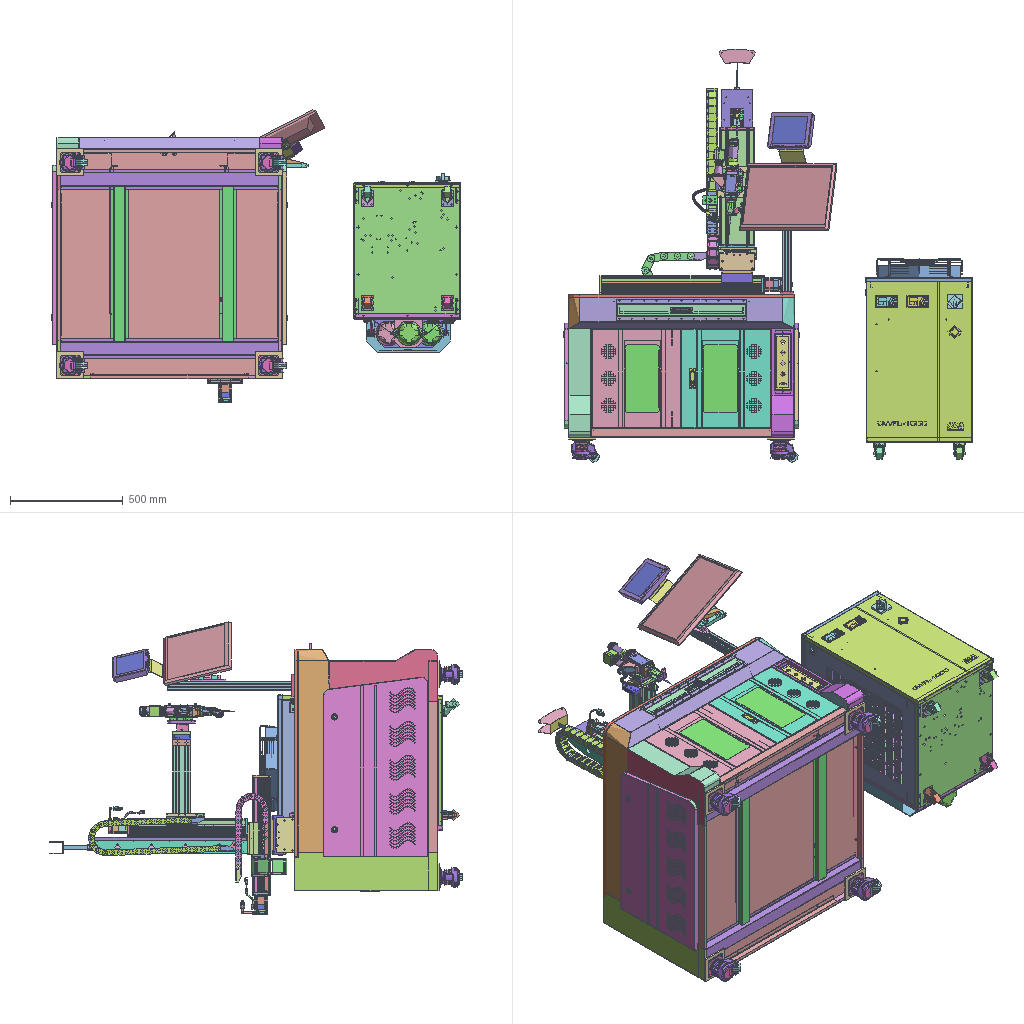Assembly | STEP file | 293 different items | 588 placed | box 1817 x 1832 x 1296 mm
Parts list (item | name | quantity | parent item | size | volume):
1 | FHD-021-001-A rack welded part A | x1 | in BHB-002-000-001 rack welding | 1000 x 1020 x 40 mm | 1755209 mm3
2 | FHD-021-001-B rack welded part B | x1 | in BHB-002-000-001 rack welding | 1000 x 198.5 x 167.5 mm | 523284 mm3
3 | FHD-021-001-C rack welded part C | x1 | in BHB-002-000-001 rack welding | 633.5 x 171.5 x 165 mm | 350229 mm3
4 | FHD-021-001-D rack welded part D | x1 | in BHB-002-000-001 rack welding | 633.5 x 165 x 171.5 mm | 312915 mm3
5 | FHD-021-001-E rack welded part E | x1 | in BHB-002-000-001 rack welding | 900 x 139 x 50 mm | 280758 mm3
6 | FHD-021-001-F rack welded part F | x1 | in BHB-002-000-001 rack welding | 900 x 139 x 50 mm | 288308 mm3
7 | FHD-021-001-G rack welded part G | x1 | in BHB-002-000-001 rack welding | 1000 x 178.631 x 144.83 mm | 461158 mm3
8 | FHD-021-001-H rack welded part H | x1 | in BHB-002-000-001 rack welding | 483 x 230 x 20 mm | 162335 mm3
9 | FHD-021-001-I rack welded part I | x1 | in BHB-002-000-001 rack welding | 483 x 230 x 20 mm | 162335 mm3
10 | FHD-021-001-J rack welded part J | x1 | in BHB-002-000-001 rack welding | 482.9 x 130.5 x 173 mm | 174985 mm3
11 | FHD-021-001-K rack welded part K | x1 | in BHB-002-000-001 rack welding | 482.9 x 126.5 x 173 mm | 173847 mm3
12 | FHD-021-001-L rack welded part L | x1 | in BHB-002-000-001 rack welding | 480.9 x 65 x 100 mm | 53460 mm3
13 | FHD-021-001-M rack welded part M | x1 | in BHB-002-000-001 rack welding | 480.9 x 65 x 100 mm | 79687 mm3
14 | FHD-021-001-N rack welded part N | x2 | in BHB-002-000-001 rack welding | 30 x 73.5 x 446.5 mm | 80480 mm3
15 | FHD-021-001-O rack welded part O | x2 | in BHB-002-000-001 rack welding | 20 x 73.5 x 446.5 mm | 91052 mm3
16 | FHD-021-001-P rack welded part P | x2 | in BHB-002-000-001 rack welding | 1000 x 80 x 15 mm | 159142 mm3
17 | FHD-021-001-Q rack welded part Q | x1 | in BHB-002-000-001 rack welding | 280 x 73 x 20 mm | 29608 mm3
18 | FHD-021-001-R rack welded part R | x1 | in BHB-002-000-001 rack welding | 244 x 74 x 1.5 mm | 11328 mm3
19 | FHD-021-001-Z Fuma wheel mounting plate | x4 | in BHB-002-000-001 rack welding | 120 x 120 x 8 mm | 114038 mm3
20 | FHD-021-001-S rack welded part S | x2 | in BHB-002-000-001 rack welding | 969 x 87 x 38.5 mm | 231643 mm3
21 | FHD-021-001-T rack welded part T | x2 | in BHB-002-000-001 rack welding | 690 x 77 x 20 mm | 115059 mm3
22 | FHD-021-001-U rack welded part U | x1 | in BHB-002-000-001 rack welding | 336.5 x 121.5 x 15 mm | 72345 mm3
23 | FHD-021-001-V rack welded part V | x1 | in BHB-002-000-001 rack welding | 336.5 x 121.5 x 15 mm | 72345 mm3
24 | FHD-021-001-W rack welded part W | x2 | in BHB-002-000-001 rack welding | 575 x 20 x 15 mm | 28039 mm3
25 | FHD-021-001-X rack welded part X | x1 | in BHB-002-000-001 rack welding | 143 x 80 x 15 mm | 22271 mm3
26 | FHD-021-001-Y rack welded part Y | x1 | in BHB-002-000-001 rack welding | 146 x 60 x 15 mm | 27524 mm3
27 | FHD-021-002 electrical mounting plate | x2 | in FHD-021-000 H1010 cabinet | 650 x 440 x 15 mm | 470822 mm3
28 | FHD-021-003 rear door lower crossbeam | x1 | in FHD-021-000 H1010 cabinet | 695 x 103 x 22 mm | 152226 mm3
29 | FHD-021-004-A rear door A | x1 | in FHD-021-004 rear door welded body | 693 x 376 x 18 mm | 424515 mm3
30 | FHD-021-004-B fan support cover | x4 | in FHD-021-004 rear door welded body | 139 x 132 x 7 mm | 12460 mm3
31 | FHD-021-004-C rear door reinforcing rib | x1 | in FHD-021-004 rear door welded body | 348 x 57 x 10 mm | 37777 mm3
32 | FHD-021-005 power button plate | x1 | in FHD-021-000 H1010 cabinet | 248 x 68 x 1.5 mm | 22504 mm3
33 | FHD-021-006 rear power board | x1 | in FHD-021-000 H1010 cabinet | 228.5 x 58.5 x 3.2 mm | 14630 mm3
34 | FHD-021-007-A TZD10S drawer 1 | x1 | in FHD-021-007 TZD10S drawer assembly | 569.6 x 52 x 18 mm | 67956 mm3
35 | FHD-021-007-B TZD10S drawer 2 | x1 | in FHD-021-007 TZD10S drawer assembly | 548 x 320 x 25 mm | 247788 mm3
36 | FHD-021-007-C TZD10S drawer 3 | x2 | in FHD-021-007 TZD10S drawer assembly | 52 x 18 x 12 mm | 1523 mm3
37 | FHD-021-007-D TZD10S drawer 4 | x1 | in FHD-021-007 TZD10S drawer assembly | 150 x 90 x 35 mm | 35026 mm3
38 | LS707 rotary concealed handle | x2 | in FHD-021-007 TZD10S drawer assembly, FHD-021-000 H1010 cabinet | 63.292 x 100 x 20 mm | 9779 mm3
39 | FHD-021-008-01-A circuit breaker bracket 1 | x1 | in FHD-021-008-01 circuit breaker bracket welding | 100 x 108 x 20 mm | 20485 mm3
40 | FHD-021-008-01-B circuit breaker bracket 2 | x2 | in FHD-021-008-01 circuit breaker bracket welding | 57 x 47 x 15 mm | 5499 mm3
41 | FHD-021-008-01-C circuit breaker bracket 3 | x2 | in FHD-021-008-01 circuit breaker bracket welding | 76 x 20 x 1.5 mm | 2280 mm3
42 | FHD-021-008-02 limit block | x2 | in FHD-021-008 circuit breaker assembly | 60 x 70 x 19 mm | 6672 mm3
43 | FHD-021-008-03 fixing plate | x1 | in FHD-021-008 circuit breaker assembly | 103 x 25 x 1.5 mm | 3776 mm3
44 | FHD-021-009 front baffle | x2 | in FHD-021-000 H1010 cabinet | 215 x 35 x 2 mm | 14477 mm3
45 | door lock catch | x2 | in MS603 red spring door lock, MS603 red spring door lock_2 | 26.4 x 86 x 16.7 mm | 21050 mm3
46 | door lock bent plate | x2 | in MS603 red spring door lock, MS603 red spring door lock_2 | 65.681 x 31 x 12.394 mm | 2703 mm3
47 | slide rail 300-1 | x2 | in 12-inch silent slide rail, 12-inch silent slide rail_2 | 300 x 46.341 x 13 mm | 22910 mm3
48 | slide rail 300-2 | x2 | in 12-inch silent slide rail, 12-inch silent slide rail_2 | 10.373 x 34.385 x 300 mm | 15280 mm3
49 | slide rail 300-3 | x2 | in 12-inch silent slide rail, 12-inch silent slide rail_2 | 9.001 x 23.751 x 300 mm | 9128 mm3
50 | FHD-021-010 L-shaped support rail | x1 | in FHD-021-000 H1010 cabinet | 620 x 30 x 50 mm | 94894 mm3
51 | FHD-021-011-A side door A | x1 | in FHD-021-011 side door A welded body | 795.88 x 474.5 x 40 mm | 624851 mm3
52 | FHD-021-012-B side door A-B | x2 | in FHD-021-011 side door A welded body, FHD-021-012 side door B welded body | 29.753 x 26.353 x 17 mm | 1076 mm3
53 | FHD-021-012-C side door A-C | x2 | in FHD-021-011 side door A welded body, FHD-021-012 side door B welded body | 30 x 33.839 x 17 mm | 1267 mm3
54 | FHD-021-012-D side door A-D | x2 | in FHD-021-011 side door A welded body, FHD-021-012 side door B welded body | 29.753 x 27.697 x 1.5 mm | 623.148 mm3
55 | FHD-021-012-F side door A-E | x2 | in FHD-021-011 side door A welded body, FHD-021-012 side door B welded body | 30 x 33.839 x 1.5 mm | 734.02 mm3
56 | FHD-0210-012-E side door A-F | x2 | in FHD-021-011 side door A welded body, FHD-021-012 side door B welded body | 757 x 71 x 12 mm | 102614 mm3
57 | FHD-021-012-A side door B | x1 | in FHD-021-012 side door B welded body | 795.88 x 474.5 x 40 mm | 624852 mm3
58 | FHD-021-013-A front door A | x1 | in FHD-021-013-01 front door A welding | 397 x 457.5 x 17.5 mm | 250425 mm3
59 | FHD-021-014-C acrylic mounting strip | x4 | in FHD-021-013-01 front door A welding, FHD-021-014-01 front door B welding | 430 x 20 x 10 mm | 23632 mm3
60 | FHD-021-014-02 acrylic press plate | x4 | in FHD-021-013 front door A, FHD-021-014 front door B welded body | 250 x 28 x 7 mm | 12276 mm3
61 | FHD-021-014-03 acrylic | x2 | in FHD-021-013 front door A, FHD-021-014 front door B welded body | 385 x 160 x 5 mm | 308000 mm3
62 | FHD-021-014-A front door B | x1 | in FHD-021-014-01 front door B welding | 410 x 447 x 20 mm | 253871 mm3
63 | FHD-021-014-B latch mounting seat | x2 | in FHD-021-014-01 front door B welding | 70 x 40 x 15 mm | 6920 mm3
64 | latch | x2 | in LS406 automatic spring latch, LS406 automatic spring latch_2 | 30 x 13 x 66 mm | 12946 mm3
65 | latch post | x2 | in LS406 automatic spring latch, LS406 automatic spring latch_2 | 16 x 83 x 14 mm | 4581 mm3
66 | MS705-18 triangular lock core | x4 | in FHD-021-000 H1010 cabinet | 28 x 32 x 60.591 mm | 12821 mm3
67 | FHD-021-015 H1010 revised work panel | x1 | in FHD-021-000 H1010 cabinet | 1000 x 918 x 15 mm | 13697706 mm3
68 | - | x4 | in GD-80-F Fuma(2)^GD-80-F Fuma, GD-80-F Fuma(2)^GD-80-F Fuma_2, GD-80-F Fuma(2)^GD-80-F Fuma_3, GD-80-F Fuma(2)^GD-80-F Fuma_4 | 9.62 x 9.62 x 8 mm | 49.009 mm3
69 | - | x4 | in GD-80-F Fuma(2)^GD-80-F Fuma, GD-80-F Fuma(2)^GD-80-F Fuma_2, GD-80-F Fuma(2)^GD-80-F Fuma_3, GD-80-F Fuma(2)^GD-80-F Fuma_4 | 7.817 x 18 x 5 mm | 4.038 mm3
70 | - | x4 | in GD-80-F Fuma(2)^GD-80-F Fuma, GD-80-F Fuma(2)^GD-80-F Fuma_2, GD-80-F Fuma(2)^GD-80-F Fuma_3, GD-80-F Fuma(2)^GD-80-F Fuma_4 | 90 x 90 x 88.64 mm | 185053 mm3
71 | - | x4 | in GD-80-F Fuma(2)^GD-80-F Fuma, GD-80-F Fuma(2)^GD-80-F Fuma_2, GD-80-F Fuma(2)^GD-80-F Fuma_3, GD-80-F Fuma(2)^GD-80-F Fuma_4 | 63 x 32 x 63 mm | 83090 mm3
72 | - | x4 | in GD-80-F Fuma(2)^GD-80-F Fuma, GD-80-F Fuma(2)^GD-80-F Fuma_2, GD-80-F Fuma(2)^GD-80-F Fuma_3, GD-80-F Fuma(2)^GD-80-F Fuma_4 | 27.164 x 61.45 x 3.959 mm | 161.362 mm3
73 | - | x4 | in GD-80-F Fuma(2)^GD-80-F Fuma, GD-80-F Fuma(2)^GD-80-F Fuma_2, GD-80-F Fuma(2)^GD-80-F Fuma_3, GD-80-F Fuma(2)^GD-80-F Fuma_4 | 110.5 x 86 x 80.5 mm | 156144 mm3
74 | - | x1 | - | 3 x 5.5 x 5.5 mm | 47.924 mm3
75 | - | x1 | - | 6 x 6 x 0.5 mm | 10.116 mm3
76 | - | x1 | - | 3 x 5.5 x 5.5 mm | 47.924 mm3
77 | - | x1 | - | 6 x 6 x 0.5 mm | 10.116 mm3
78 | - | x1 | - | 3 x 5.5 x 5.5 mm | 47.924 mm3
79 | - | x1 | - | 6 x 6 x 0.5 mm | 10.116 mm3
80 | - | x1 | - | 3 x 5.5 x 5.5 mm | 47.924 mm3
81 | - | x1 | - | 6 x 6 x 0.5 mm | 10.116 mm3
82 | - | x1 | - | 3 x 5.5 x 5.5 mm | 47.924 mm3
83 | - | x1 | - | 6 x 6 x 0.5 mm | 10.116 mm3
84 | - | x1 | - | 3 x 5.5 x 5.5 mm | 47.924 mm3
85 | - | x1 | - | 6 x 6 x 0.5 mm | 10.116 mm3
86 | - | x1 | - | 3 x 5.5 x 5.5 mm | 47.924 mm3
87 | - | x1 | - | 6 x 6 x 0.5 mm | 10.116 mm3
88 | - | x1 | - | 3 x 5.5 x 5.5 mm | 47.924 mm3
89 | - | x1 | - | 6 x 6 x 0.5 mm | 10.116 mm3
90 | - | x1 | - | 2.7 x 4.5 x 4.5 mm | 28.373 mm3
91 | - | x1 | - | 5.2 x 5.179 x 0.6 mm | 8.765 mm3
92 | - | x1 | - | 5 x 5 x 0.5 mm | 6.955 mm3
93 | - | x1 | - | 2.7 x 4.5 x 4.5 mm | 28.373 mm3
94 | - | x1 | - | 5.2 x 5.179 x 0.6 mm | 8.765 mm3
95 | - | x1 | - | 5 x 5 x 0.5 mm | 6.955 mm3
96 | - | x1 | - | 60 x 60 x 34.1 mm | 106428 mm3
97 | - | x1 | - | 59.4 x 59.4 x 23.3 mm | 72108 mm3
98 | - | x1 | - | 60 x 60 x 6.4 mm | 20143 mm3
99 | - | x1 | - | 59.8 x 59.8 x 0.5 mm | 1478 mm3
100 | - | x1 | - | 59.8 x 64.9 x 13.2 mm | 38412 mm3
101 | - | x1 | - | 30 x 8.8 x 21 mm | 202.601 mm3
102 | - | x1 | - | 30 x 12.5 x 21 mm | 6057 mm3
103 | - | x1 | - | 10.4 x 42.4 x 119.7 mm | 5288 mm3
104 | - | x1 | - | 58.9 x 42.4 x 59.5 mm | 11878 mm3
105 | - | x1 | - | 10.6 x 6.6 x 10.6 mm | 286.348 mm3
106 | - | x1 | - | 13.2 x 8.2 x 13.2 mm | 283.542 mm3
107 | - | x1 | - | 60.2 x 60.2 x 9.5 mm | 18131 mm3
108 | - | x1 | - | 35 x 10 x 35 mm | 6585 mm3
109 | - | x1 | - | 17 x 17 x 80.2 mm | 12671 mm3
110 | - | x4 | - | 2.5 x 2.5 x 10 mm | 49.087 mm3
111 | - | x1 | - | 5 x 5 x 14 mm | 350 mm3
112 | - | x1 | - | 155 x 59.25 x 710 mm | 2291681 mm3
113 | - | x1 | - | 170 x 42.5 x 140 mm | 521938 mm3
114 | - | x1 | - | 155 x 25 x 709.4 mm | 387813 mm3
115 | - | x1 | - | 49 x 39.6 x 50 mm | 57288 mm3
116 | - | x1 | - | 155 x 82 x 12 mm | 118532 mm3
117 | - | x1 | - | 155 x 82 x 10 mm | 121887 mm3
118 | - | x2 | - | 15 x 15 x 700 mm | 150376 mm3
119 | - | x1 | - | 69.5 x 46 x 22 mm | 45024 mm3
120 | - | x1 | - | 69.5 x 49 x 25 mm | 41553 mm3
121 | - | x1 | - | 16 x 16 x 675 mm | 128698 mm3
122 | - | x4 | - | 56 x 33 x 16 mm | 20352 mm3
123 | - | x1 | - | 40 x 30 x 10 mm | 9671 mm3
124 | - | x1 | in X-axis module | 170 x 140 x 12 mm | 282154 mm3
125 | - | x2 | in module drag chain72X35assemblyX500 stroke | 104 x 72 x 35 mm | 42394 mm3
126 | - | x14 | in module drag chain72X35assemblyX500 stroke | 94 x 35 x 72 mm | 47784 mm3
127 | - | x1 | - | 15 x 15 x 500 mm | 107236 mm3
128 | - | x2 | - | 56 x 33 x 16 mm | 20352 mm3
129 | - | x1 | - | 15 x 15 x 500 mm | 107236 mm3
130 | - | x2 | - | 56 x 33 x 16 mm | 20352 mm3
131 | - | x1 | - | 3 x 5.5 x 5.5 mm | 47.924 mm3
132 | - | x1 | - | 6 x 6 x 0.5 mm | 10.116 mm3
133 | - | x1 | - | 3 x 5.5 x 5.5 mm | 47.924 mm3
134 | - | x1 | - | 6 x 6 x 0.5 mm | 10.116 mm3
135 | - | x1 | - | 3 x 5.5 x 5.5 mm | 47.924 mm3
136 | - | x1 | - | 6 x 6 x 0.5 mm | 10.116 mm3
137 | - | x1 | - | 3 x 5.5 x 5.5 mm | 47.924 mm3
138 | - | x1 | - | 6 x 6 x 0.5 mm | 10.116 mm3
139 | - | x1 | - | 3 x 5.5 x 5.5 mm | 47.924 mm3
140 | - | x1 | - | 6 x 6 x 0.5 mm | 10.116 mm3
141 | - | x1 | - | 3 x 5.5 x 5.5 mm | 47.924 mm3
142 | - | x1 | - | 6 x 6 x 0.5 mm | 10.116 mm3
143 | - | x1 | - | 3 x 5.5 x 5.5 mm | 47.924 mm3
144 | - | x1 | - | 6 x 6 x 0.5 mm | 10.116 mm3
145 | - | x1 | - | 3 x 5.5 x 5.5 mm | 47.924 mm3
146 | - | x1 | - | 6 x 6 x 0.5 mm | 10.116 mm3
147 | - | x1 | - | 2.7 x 4.5 x 4.5 mm | 28.373 mm3
148 | - | x1 | - | 5.2 x 5.179 x 0.6 mm | 8.765 mm3
149 | - | x1 | - | 5 x 5 x 0.5 mm | 6.955 mm3
150 | - | x1 | - | 2.7 x 4.5 x 4.5 mm | 28.373 mm3
151 | - | x1 | - | 5.2 x 5.179 x 0.6 mm | 8.765 mm3
152 | - | x1 | - | 5 x 5 x 0.5 mm | 6.955 mm3
153 | - | x1 | - | 60 x 60 x 34.1 mm | 106428 mm3
154 | - | x1 | - | 59.4 x 59.4 x 23.3 mm | 72108 mm3
155 | - | x1 | - | 60 x 60 x 6.4 mm | 20143 mm3
156 | - | x1 | - | 59.8 x 59.8 x 0.5 mm | 1478 mm3
157 | - | x1 | - | 59.8 x 64.9 x 13.2 mm | 38412 mm3
158 | - | x1 | - | 30 x 8.8 x 21 mm | 202.601 mm3
159 | - | x1 | - | 30 x 12.5 x 21 mm | 6057 mm3
160 | - | x1 | - | 10.4 x 42.4 x 119.7 mm | 5288 mm3
161 | - | x1 | - | 58.9 x 42.4 x 59.5 mm | 11878 mm3
162 | - | x1 | - | 10.6 x 6.6 x 10.6 mm | 286.348 mm3
163 | - | x1 | - | 13.2 x 8.2 x 13.2 mm | 283.542 mm3
164 | - | x1 | - | 60.2 x 60.2 x 9.5 mm | 18131 mm3
165 | - | x1 | - | 35 x 10 x 35 mm | 6585 mm3
166 | - | x1 | - | 17 x 17 x 80.2 mm | 12671 mm3
167 | - | x4 | - | 2.5 x 2.5 x 10 mm | 49.087 mm3
168 | - | x1 | - | 5 x 5 x 14 mm | 350 mm3
169 | - | x1 | - | 475 x 15 x 15 mm | 78728 mm3
170 | - | x1 | - | 10 x 15 x 15 mm | 632.723 mm3
171 | - | x1 | - | 38 x 48 x 40 mm | 23611 mm3
172 | - | x1 | - | 155 x 59.25 x 510 mm | 1638081 mm3
173 | - | x1 | - | 49 x 39.6 x 50 mm | 57288 mm3
174 | - | x1 | - | 170 x 42.5 x 140 mm | 522527 mm3
175 | - | x1 | - | 155 x 25 x 509.4 mm | 278478 mm3
176 | - | x1 | - | 155 x 82 x 12 mm | 118532 mm3
177 | - | x1 | - | 155 x 82 x 10 mm | 121887 mm3
178 | - | x1 | - | 69.5 x 46 x 22 mm | 45024 mm3
179 | - | x1 | - | 69.5 x 49 x 25 mm | 41553 mm3
180 | - | x1 | - | 38 x 11 x 30 mm | 9809 mm3
181 | - | x2 | - | 12 x 14 x 12 mm | 1266 mm3
182 | - | x1 | - | 8 x 26 x 26 mm | 3460 mm3
183 | - | x1 | - | 54 x 54 x 34.8 mm | 31485 mm3
184 | - | x1 | - | 28 x 28 x 32 mm | 13816 mm3
185 | - | x1 | - | 5 x 11.9 x 37.5 mm | 433.441 mm3
186 | - | x2 | - | 13.4 x 41 x 12 mm | 1188 mm3
187 | - | x48 | - | 20 x 7 x 7 mm | 335.507 mm3
188 | - | x10 | - | 21 x 8.5 x 8.5 mm | 554.949 mm3
189 | - | x4 | - | 11 x 5.5 x 5.5 mm | 118.766 mm3
190 | - | x16 | - | 25 x 8.5 x 8.5 mm | 633.488 mm3
191 | - | x1 | - | 12.9 x 14.3 x 1 mm | 65.231 mm3
192 | - | x1 | in Y-axis module | 300 x 60 x 32 mm | 62070 mm3
193 | - | x1 | in Y-axis module | 100 x 72 x 35 mm | 19846 mm3
194 | - | x2 | - | 80 x 48 x 25 mm | 22611 mm3
195 | - | x17 | - | 58.5 x 25 x 48 mm | 18741 mm3
196 | - | x2 | - | 60 x 700 x 15 mm | 546170 mm3
197 | - | x1 | - | 170 x 140 x 12 mm | 277366 mm3
198 | - | x1 | - | 700 x 140 x 15 mm | 1462585 mm3
199 | - | x1 | - | 60 x 58 x 60 mm | 38921 mm3
200 | - | x2 | - | 1.5 x 159.863 x 63.96 mm | 12341 mm3
201 | - | x1 | - | 20 x 20 x 700 mm | 96209 mm3
202 | - | x1 | - | 50 x 106.693 x 5.46 mm | 7969 mm3
203 | - | x1 | - | 28 x 25 x 700 mm | 101372 mm3
204 | - | x1 | - | 15 x 15 x 500 mm | 107236 mm3
205 | - | x2 | - | 56 x 33 x 16 mm | 20352 mm3
206 | - | x1 | - | 15 x 15 x 500 mm | 107236 mm3
207 | - | x2 | - | 56 x 33 x 16 mm | 20352 mm3
208 | - | x1 | - | 3 x 5.5 x 5.5 mm | 47.924 mm3
209 | - | x1 | - | 6 x 6 x 0.5 mm | 10.116 mm3
210 | - | x1 | - | 3 x 5.5 x 5.5 mm | 47.924 mm3
211 | - | x1 | - | 6 x 6 x 0.5 mm | 10.116 mm3
212 | - | x1 | - | 3 x 5.5 x 5.5 mm | 47.924 mm3
213 | - | x1 | - | 6 x 6 x 0.5 mm | 10.116 mm3
214 | - | x1 | - | 3 x 5.5 x 5.5 mm | 47.924 mm3
215 | - | x1 | - | 6 x 6 x 0.5 mm | 10.116 mm3
216 | - | x1 | - | 3 x 5.5 x 5.5 mm | 47.924 mm3
217 | - | x1 | - | 6 x 6 x 0.5 mm | 10.116 mm3
218 | - | x1 | - | 3 x 5.5 x 5.5 mm | 47.924 mm3
219 | - | x1 | - | 6 x 6 x 0.5 mm | 10.116 mm3
220 | - | x1 | - | 3 x 5.5 x 5.5 mm | 47.924 mm3
221 | - | x1 | - | 6 x 6 x 0.5 mm | 10.116 mm3
222 | - | x1 | - | 3 x 5.5 x 5.5 mm | 47.924 mm3
223 | - | x1 | - | 6 x 6 x 0.5 mm | 10.116 mm3
224 | - | x1 | - | 2.7 x 4.5 x 4.5 mm | 28.373 mm3
225 | - | x1 | - | 5.2 x 5.179 x 0.6 mm | 8.765 mm3
226 | - | x1 | - | 5 x 5 x 0.5 mm | 6.955 mm3
227 | - | x1 | - | 2.7 x 4.5 x 4.5 mm | 28.373 mm3
228 | - | x1 | - | 5.2 x 5.179 x 0.6 mm | 8.765 mm3
229 | - | x1 | - | 5 x 5 x 0.5 mm | 6.955 mm3
230 | - | x1 | - | 60 x 60 x 34.1 mm | 106428 mm3
231 | - | x1 | - | 59.4 x 59.4 x 23.3 mm | 72108 mm3
232 | - | x1 | - | 60 x 60 x 6.4 mm | 20143 mm3
233 | - | x1 | - | 59.8 x 59.8 x 0.5 mm | 1478 mm3
234 | - | x1 | - | 59.8 x 64.9 x 13.2 mm | 38412 mm3
235 | - | x1 | - | 30 x 8.8 x 21 mm | 202.601 mm3
236 | - | x1 | - | 30 x 12.5 x 21 mm | 6057 mm3
237 | - | x1 | - | 10.4 x 42.4 x 119.7 mm | 5288 mm3
238 | - | x1 | - | 58.9 x 42.4 x 59.5 mm | 11878 mm3
239 | - | x1 | - | 10.6 x 6.6 x 10.6 mm | 286.348 mm3
240 | - | x1 | - | 13.2 x 8.2 x 13.2 mm | 283.542 mm3
241 | - | x1 | - | 60.2 x 60.2 x 9.5 mm | 18131 mm3
242 | - | x1 | - | 35 x 10 x 35 mm | 6585 mm3
243 | - | x1 | - | 17 x 17 x 80.2 mm | 12671 mm3
244 | - | x4 | - | 2.5 x 2.5 x 10 mm | 49.087 mm3
245 | - | x1 | - | 5 x 5 x 14 mm | 350 mm3
246 | - | x1 | - | 475 x 15 x 15 mm | 78728 mm3
247 | - | x1 | - | 10 x 15 x 15 mm | 632.723 mm3
248 | - | x1 | - | 38 x 48 x 40 mm | 23611 mm3
249 | - | x1 | - | 155 x 59.25 x 510 mm | 1638081 mm3
250 | - | x1 | - | 49 x 39.6 x 50 mm | 57288 mm3
251 | - | x1 | - | 170 x 42.5 x 140 mm | 522527 mm3
252 | - | x1 | - | 155 x 25 x 509.4 mm | 278478 mm3
253 | - | x1 | - | 155 x 82 x 12 mm | 118532 mm3
254 | - | x1 | - | 155 x 82 x 10 mm | 121887 mm3
255 | - | x1 | - | 69.5 x 46 x 22 mm | 45024 mm3
256 | - | x1 | - | 69.5 x 49 x 25 mm | 41553 mm3
257 | - | x1 | - | 38 x 11 x 30 mm | 9809 mm3
258 | - | x2 | - | 12 x 14 x 12 mm | 1266 mm3
259 | - | x1 | - | 8 x 26 x 26 mm | 3460 mm3
260 | - | x1 | - | 54 x 54 x 34.8 mm | 31485 mm3
261 | - | x1 | - | 28 x 28 x 32 mm | 13816 mm3
262 | - | x1 | - | 5 x 11.9 x 37.5 mm | 433.441 mm3
263 | - | x2 | - | 13.4 x 41 x 12 mm | 1188 mm3
264 | - | x48 | - | 20 x 7 x 7 mm | 335.507 mm3
265 | - | x10 | - | 21 x 8.5 x 8.5 mm | 554.949 mm3
266 | - | x4 | - | 11 x 5.5 x 5.5 mm | 118.766 mm3
267 | - | x16 | - | 25 x 8.5 x 8.5 mm | 633.488 mm3
268 | - | x1 | - | 12.9 x 14.3 x 1 mm | 65.231 mm3
269 | - | x1 | - | 80 x 80 x 350 mm | 477520 mm3
270 | - | x1 | - | 80 x 50 x 14 mm | 51452 mm3
271 | - | x1 | - | 80 x 40 x 20 mm | 53799 mm3
272 | - | x1 | - | 80 x 80 x 15 mm | 88507 mm3
273 | - | x1 | - | 58 x 50 x 30 mm | 56140 mm3
274 | - | x1 | - | 36 x 36 x 35 mm | 25571 mm3
275 | - | x1 | - | 170 x 140 x 12 mm | 277063 mm3
276 | - | x1 | - | 120 x 90 x 12 mm | 121667 mm3
277 | - | x1 | in Z-axis module | 68 x 40 x 15 mm | 6435 mm3
278 | - | x1 | in Z-axis module | 76 x 36 x 47 mm | 12306 mm3
279 | module 48X25 drag chainA | x2 | in module 48X25 drag chainB | 80 x 48 x 25 mm | 22611 mm3
280 | module 48X25 drag chainA2 | x32 | in module 48X25 drag chainB | 58.5 x 25 x 48 mm | 18741 mm3
281 | XHG200AYH(F100-F200) | x1 | in welding head moving assembly | - | -
282 | - | x1 | - | 60.601 x 162 x 27 mm | 75887 mm3
283 | - | x2 | - | 20 x 160 x 29 mm | 68270 mm3
284 | - | x1 | - | 128 x 18 x 30 mm | 60581 mm3
285 | - | x1 | - | 41.5 x 23 x 23 mm | 10947 mm3
286 | - | x1 | - | 116 x 116 x 45 mm | 39889 mm3
287 | - | x1 | in monitor stand BPB-037-000 monitor column mounting assembly(2)^BPB-037-000 monitor column mounting assembly | 100 x 12 x 60 mm | 66467 mm3
288 | - | x1 | in monitor stand BPB-037-000 monitor column mounting assembly(2)^BPB-037-000 monitor column mounting assembly | 40 x 550 x 40 mm | 261689 mm3
289 | - | x1 | in monitor stand BPB-037-000 monitor column mounting assembly(2)^BPB-037-000 monitor column mounting assembly | 447.598 x 120 x 42.426 mm | 103118 mm3
290 | - | x1 | in monitor stand BPB-037-000 monitor column mounting assembly(2)^BPB-037-000 monitor column mounting assembly | 40 x 10.5 x 40 mm | 4637 mm3
291 | HJ0101000A0 CCD display model | x1 | in monitor stand BPB-037-000 monitor column mounting assembly(2)^BPB-037-000 monitor column mounting assembly | 204 x 163 x 37.5 mm | 989261 mm3
292 | computer monitor | x1 | in monitor stand BPB-037-000 monitor column mounting assembly(2)^BPB-037-000 monitor column mounting assembly | 440 x 308.73 x 50 mm | 3953854 mm3
293 | chiller 506 CWFL-1500 shell | x1 | - | - | -
Placements (level | parent | child | x y z in mm | rotation matrix by rows), first 272 of 672 lines:
1 | subassembly 2 | FHD-021-000 H1010 closed cabinet (no cover) | 195.342 -389.886 1540.341 | 1 0 0 0 0 1 0 -1 0
2 | FHD-021-000 H1010 closed cabinet (no cover) | FHD-021-000 H1010 cabinet | -0.0 -0.0 -0.0 | 1 0 0 0 1 0 0 0 1
3 | FHD-021-000 H1010 cabinet | FHD-021-001 H1010 cabinet | -99.946 64.846 -213.742 | 1 0 0 0 1 0 0 0 1
4 | FHD-021-001 H1010 cabinet | BHB-002-000-001 rack welding | -0.0 -0.0 -0.0 | 1 0 0 0 1 0 0 0 1
5 | BHB-002-000-001 rack welding | FHD-021-001-A rack welded part A | -9.957 5.221 20.0 | 1 0 0 0 1 0 0 0 1
5 | BHB-002-000-001 rack welding | FHD-021-001-B rack welded part B | -9.957 440.221 615.0 | -1 0 0 0 -1 0 0 0 1
5 | BHB-002-000-001 rack welding | FHD-021-001-C rack welded part C | -509.957 430.221 297.5 | 0 0 -1 0 -1 0 -1 0 -0
5 | BHB-002-000-001 rack welding | FHD-021-001-D rack welded part D | 415.043 515.221 297.5 | 0 -1 0 0 0 1 -1 0 0
5 | BHB-002-000-001 rack welding | FHD-021-001-E rack welded part E | 490.043 -104.779 529.75 | 0 0 1 1 0 0 0 1 0
5 | BHB-002-000-001 rack welding | FHD-021-001-F rack welded part F | -509.957 -104.779 529.75 | 0 0 -1 -1 0 0 0 1 0
5 | BHB-002-000-001 rack welding | FHD-021-001-G rack welded part G | -2082.417 5624.075 -3076.863 | 1 0 0 0 -0.866 -0.5 0 0.5 -0.866
5 | BHB-002-000-001 rack welding | FHD-021-001-H rack welded part H | 490.043 -439.779 220.5 | 0 0 1 0 1 0 -1 0 0
5 | BHB-002-000-001 rack welding | FHD-021-001-I rack welded part I | -508.457 -439.779 220.5 | 0 0 1 0 1 0 -1 0 0
5 | BHB-002-000-001 rack welding | FHD-021-001-J rack welded part J | 391.543 -519.029 220.45 | 0 0 1 0 1 0 -1 0 0
5 | BHB-002-000-001 rack welding | FHD-021-001-K rack welded part K | -409.957 -519.029 220.45 | 0 0 1 0 1 0 -1 0 0
5 | BHB-002-000-001 rack welding | FHD-021-001-L rack welded part L | 440.043 -504.779 460.9 | 0 0 1 0 1 0 -1 0 0
5 | BHB-002-000-001 rack welding | FHD-021-001-M rack welded part M | -459.957 -504.779 460.9 | 0 0 1 0 1 0 -1 0 0
5 | BHB-002-000-001 rack welding | FHD-021-001-N rack welded part N | -238.457 -428.279 241.25 | 1 0 0 0 1 0 0 0 1
5 | BHB-002-000-001 rack welding | FHD-021-001-N rack welded part N | 218.543 -428.279 241.25 | -1 0 0 0 1 0 0 0 -1
5 | BHB-002-000-001 rack welding | FHD-021-001-O rack welded part O | 218.543 226.721 241.25 | -1 0 0 0 -1 0 0 0 1
5 | BHB-002-000-001 rack welding | FHD-021-001-O rack welded part O | -238.457 226.721 241.25 | 1 0 0 0 -1 0 0 0 -1
5 | BHB-002-000-001 rack welding | FHD-021-001-P rack welded part P | 237.543 13.721 463.941 | 0 -1 0 1 0 0 0 0 1
5 | BHB-002-000-001 rack welding | FHD-021-001-P rack welded part P | -257.457 13.721 463.941 | 0 -1 0 1 0 0 0 0 1
5 | BHB-002-000-001 rack welding | FHD-021-001-Q rack welded part Q | 440.043 -484.779 313.9 | 0 -1 0 0 0 -1 1 0 0
5 | BHB-002-000-001 rack welding | FHD-021-001-R rack welded part R | 415.043 513.721 120.0 | 0 -1 0 0 0 1 -1 0 0
5 | BHB-002-000-001 rack welding | FHD-021-001-Z Fuma wheel mounting plate | -449.957 -444.779 -28.0 | 0 1 0 -1 0 0 0 0 1
5 | BHB-002-000-001 rack welding | FHD-021-001-Z Fuma wheel mounting plate | 430.043 -444.779 -28.0 | 0 1 0 -1 0 0 0 0 1
5 | BHB-002-000-001 rack welding | FHD-021-001-S rack welded part S | -10.457 -369.779 -20.0 | -1 0 0 0 1 0 0 0 -1
5 | BHB-002-000-001 rack welding | FHD-021-001-S rack welded part S | -10.457 380.221 -20.0 | -1 0 0 0 1 0 0 0 -1
5 | BHB-002-000-001 rack welding | FHD-021-001-T rack welded part T | -230.889 5.221 0.0 | 0 -1 0 1 0 0 0 0 1
5 | BHB-002-000-001 rack welding | FHD-021-001-T rack welded part T | 250.006 5.221 0.0 | 0 -1 0 1 0 0 0 0 1
5 | BHB-002-000-001 rack welding | FHD-021-001-U rack welded part U | -297.457 -385.779 523.941 | 0 0 1 1 0 0 0 1 -0
5 | BHB-002-000-001 rack welding | FHD-021-001-V rack welded part V | 279.043 -385.779 523.941 | 0 0 1 1 0 0 0 1 0
5 | BHB-002-000-001 rack welding | FHD-021-001-W rack welded part W | -9.957 -553.279 582.5 | 1 0 0 0 0 -1 0 1 0
5 | BHB-002-000-001 rack welding | FHD-021-001-W rack welded part W | -9.957 -553.279 507.5 | -1 0 0 0 0 -1 0 -1 -0
5 | BHB-002-000-001 rack welding | FHD-021-001-X rack welded part X | 443.543 440.221 613.5 | 0 -1 0 1 0 0 0 0 1
5 | BHB-002-000-001 rack welding | FHD-021-001-Y rack welded part Y | 283.043 440.471 611.5 | 0 1 0 1 0 0 0 0 -1
5 | BHB-002-000-001 rack welding | FHD-021-001-Z Fuma wheel mounting plate | -449.957 455.221 -28.0 | 0 -1 0 1 0 0 0 0 1
5 | BHB-002-000-001 rack welding | FHD-021-001-Z Fuma wheel mounting plate | 430.043 455.221 -28.0 | 0 -1 0 1 0 0 0 0 1
3 | FHD-021-000 H1010 cabinet | FHD-021-002 electrical mounting plate | 153.597 -31.019 26.258 | 0 0 1 1 0 0 0 1 0
3 | FHD-021-000 H1010 cabinet | FHD-021-002 electrical mounting plate | -373.403 -31.019 26.258 | 0 0 -1 -1 0 0 0 1 -0
3 | FHD-021-000 H1010 cabinet | FHD-021-003 rear door lower crossbeam | -109.903 580.067 -152.242 | -1 0 0 0 0 1 0 1 -0
3 | FHD-021-000 H1010 cabinet | FHD-021-004 rear door welded body | -51.438 1264.075 28.256 | 1 0 0 0 0 -1 0 1 0
4 | FHD-021-004 rear door welded body | FHD-021-004-A rear door A | -57.965 39.001 685.508 | 1 0 0 0 1 0 0 0 1
4 | FHD-021-004 rear door welded body | FHD-021-004-B fan support cover | -207.965 129.001 692.508 | 1 0 0 0 1 0 0 0 1
4 | FHD-021-004 rear door welded body | FHD-021-004-B fan support cover | 92.035 129.001 692.508 | 1 0 0 0 1 0 0 0 1
4 | FHD-021-004 rear door welded body | FHD-021-004-B fan support cover | 92.035 -50.999 692.508 | 1 0 0 0 1 0 0 0 1
4 | FHD-021-004 rear door welded body | FHD-021-004-B fan support cover | -207.965 -50.999 692.508 | 1 0 0 0 1 0 0 0 1
4 | FHD-021-004 rear door welded body | FHD-021-004-C rear door reinforcing rib | -56.843 36.501 695.508 | 0 -1 0 1 0 0 0 0 1
3 | FHD-021-000 H1010 cabinet | FHD-021-005 power button plate | 340.097 -421.433 100.158 | 0 1 0 0 0 -1 -1 0 0
3 | FHD-021-000 H1010 cabinet | FHD-021-006 rear power board | 315.147 579.767 -93.742 | 0 -1 0 0 0 1 -1 0 0
3 | FHD-021-000 H1010 cabinet | FHD-021-007 TZD10S drawer assembly | -121.075 -480.933 316.808 | 1 0 0 0 0 -1 0 1 0
4 | FHD-021-007 TZD10S drawer assembly | FHD-021-007-A TZD10S drawer 1 | 11.171 14.45 9.0 | 1 0 0 0 1 0 0 0 1
4 | FHD-021-007 TZD10S drawer assembly | FHD-021-007-B TZD10S drawer 2 | 11.171 -0.35 -152.2 | 1 0 0 0 0 1 0 -1 -0
4 | FHD-021-007 TZD10S drawer assembly | FHD-021-007-C TZD10S drawer 3 | -273.629 14.45 -0.0 | 0 0 1 -1 0 0 0 -1 0
4 | FHD-021-007 TZD10S drawer assembly | FHD-021-007-C TZD10S drawer 3 | 295.971 14.45 -0.0 | 0 0 -1 1 0 0 0 -1 0
4 | FHD-021-007 TZD10S drawer assembly | FHD-021-007-D TZD10S drawer 4 | 238.971 34.65 -84.0 | 0 1 0 0 0 1 1 0 -0
4 | FHD-021-007 TZD10S drawer assembly | LS707 rotary concealed handle | 11.171 14.45 9.0 | 0 1 0 0 0 1 1 0 -0
3 | FHD-021-000 H1010 cabinet | FHD-021-008 circuit breaker assembly | -101.446 64.846 -212.242 | 1 0 0 0 1 0 0 0 1
4 | FHD-021-008 circuit breaker assembly | FHD-021-008-01 circuit breaker bracket welding | -0.0 -0.0 -0.0 | 1 0 0 0 1 0 0 0 1
5 | FHD-021-008-01 circuit breaker bracket welding | FHD-021-008-01-A circuit breaker bracket 1 | 416.543 495.221 412.0 | 1 0 0 0 0 1 0 -1 -0
5 | FHD-021-008-01 circuit breaker bracket welding | FHD-021-008-01-B circuit breaker bracket 2 | 454.543 465.221 412.0 | 0 0 1 1 0 0 0 1 -0
5 | FHD-021-008-01 circuit breaker bracket welding | FHD-021-008-01-B circuit breaker bracket 2 | 378.543 465.221 412.0 | 0 0 -1 1 0 0 0 -1 -0
5 | FHD-021-008-01 circuit breaker bracket welding | FHD-021-008-01-C circuit breaker bracket 3 | 416.543 483.721 437.0 | 1 0 0 0 1 0 0 0 1
5 | FHD-021-008-01 circuit breaker bracket welding | FHD-021-008-01-C circuit breaker bracket 3 | 416.543 483.721 388.5 | 1 0 0 0 1 0 0 0 1
4 | FHD-021-008 circuit breaker assembly | FHD-021-008-02 limit block | 415.043 466.721 412.0 | 0 0 -1 -1 0 0 0 1 0
4 | FHD-021-008 circuit breaker assembly | FHD-021-008-02 limit block | 396.543 466.721 412.0 | 0 0 -1 -1 0 0 0 1 0
4 | FHD-021-008 circuit breaker assembly | FHD-021-008-03 fixing plate | 416.543 436.721 412.0 | 1 0 0 0 0 1 0 -1 -0
3 | FHD-021-000 H1010 cabinet | FHD-021-009 front baffle | 129.514 -366.933 -83.77 | 0 1 0 0 0 -1 -1 0 0
3 | FHD-021-000 H1010 cabinet | FHD-021-009 front baffle | 129.514 -366.933 138.244 | 0 1 0 0 0 -1 -1 0 0
3 | FHD-021-000 H1010 cabinet | MS603 red spring door lock | 148.127 574.417 71.303 | -1 0 0 0 0 -1 0 -1 0
4 | MS603 red spring door lock | door lock catch | -37.469 4.545 -7.95 | 1 0 0 0 1 0 0 0 1
4 | MS603 red spring door lock | door lock bent plate | -59.546 -17.66 6.35 | 0.9998 -0.01745 0 -0.01745 -0.9998 0 0 0 -1
3 | FHD-021-000 H1010 cabinet | 12-inch silent slide rail | -616.45 -385.435 154.494 | 0 0 1 1 0 0 0 1 -0
4 | 12-inch silent slide rail | slide rail 300-1 | 112.212 171.161 219.047 | 1 0 0 0 1 0 0 0 1
4 | 12-inch silent slide rail | slide rail 300-2 | -49.498 171.477 224.858 | 0 0 1 0 1 0 -1 0 0
4 | 12-inch silent slide rail | slide rail 300-3 | -49.498 172.604 228.231 | 0 0 1 0 1 0 -1 0 0
3 | FHD-021-000 H1010 cabinet | 12-inch silent slide rail_2 | 396.644 -385.435 499.021 | 0 0 -1 1 0 0 0 -1 -0
4 | 12-inch silent slide rail_2 | slide rail 300-1 | 112.212 171.161 219.047 | 1 0 0 0 1 0 0 0 1
4 | 12-inch silent slide rail_2 | slide rail 300-2 | -49.498 171.477 224.858 | 0 0 1 0 1 0 -1 0 0
4 | 12-inch silent slide rail_2 | slide rail 300-3 | -49.498 172.604 228.231 | 0 0 1 0 1 0 -1 0 0
3 | FHD-021-000 H1010 cabinet | LS707 rotary concealed handle | -109.403 -489.933 331.258 | 0 1 0 -1 0 0 0 0 1
3 | FHD-021-000 H1010 cabinet | FHD-021-010 L-shaped support rail | 118.597 -53.433 128.494 | 0 0 1 1 0 0 0 1 0
3 | FHD-021-000 H1010 cabinet | FHD-021-011 side door A welded body | 390.099 90.395 28.479 | 0 0 1 1 0 0 0 1 -0
4 | FHD-021-011 side door A welded body | FHD-021-011-A side door A | -61.828 11.779 19.998 | 1 0 0 0 1 0 0 0 1
4 | FHD-021-011 side door A welded body | FHD-021-012-B side door A-B | 1458.877 -1046.684 18.498 | -1 0 0 0 1 0 0 0 -1
4 | FHD-021-011 side door A welded body | FHD-021-012-C side door A-C | 1458.877 -1046.684 18.498 | -1 0 0 0 1 0 0 0 -1
4 | FHD-021-011 side door A welded body | FHD-021-012-D side door A-D | 1458.877 -1046.684 -0.0019 | -1 0 0 0 1 0 0 0 -1
4 | FHD-021-011 side door A welded body | FHD-021-012-F side door A-E | 1458.877 -1046.684 -0.0019 | -1 0 0 0 1 0 0 0 -1
4 | FHD-021-011 side door A welded body | FHD-0210-012-E side door A-F | -41.828 29.572 7.998 | 1 0 0 0 1 0 0 0 1
3 | FHD-021-000 H1010 cabinet | FHD-021-012 side door B welded body | -609.905 48.479 35.765 | 0 0 1 1 0 0 0 1 0
4 | FHD-021-012 side door B welded body | FHD-021-012-A side door B | -19.912 4.493 -18.498 | 1 0 0 0 1 0 0 0 1
4 | FHD-021-012 side door B welded body | FHD-021-012-B side door A-B | 682.319 -1773.619 -18.498 | 0.128 -0.9918 0 0.9918 0.128 0 0 0 1
4 | FHD-021-012 side door B welded body | FHD-021-012-C side door A-C | -993.288 1782.605 -18.498 | -0.128 0.9918 0 -0.9918 -0.128 0 0 0 1
4 | FHD-021-012 side door B welded body | FHD-021-012-D side door A-D | 682.319 -1773.619 0.0019 | 0.128 -0.9918 0 0.9918 0.128 0 0 0 1
4 | FHD-021-012 side door B welded body | FHD-0210-012-E side door A-F | 0.0883 35.488 -7.998 | -1 0 0 0 1 0 0 0 -1
4 | FHD-021-012 side door B welded body | FHD-021-012-F side door A-E | -993.288 1782.605 0.0019 | -0.128 0.9918 0 -0.9918 -0.128 0 0 0 1
3 | FHD-021-000 H1010 cabinet | FHD-021-013 front door A | 126.497 -431.183 18.372 | -1 0 0 0 0 1 0 1 -0
4 | FHD-021-013 front door A | FHD-021-013-01 front door A welding | -0.0 -0.0 0.0 | 1 0 0 0 1 0 0 0 1
5 | FHD-021-013-01 front door A welding | FHD-021-013-A front door A | 37.4 8.136 -7.25 | 1 0 0 0 1 0 0 0 1
5 | FHD-021-013-01 front door A welding | FHD-021-014-C acrylic mounting strip | 157.9 5.886 1.25 | 0 -1 0 -1 0 0 0 0 -1
5 | FHD-021-013-01 front door A welding | FHD-021-014-C acrylic mounting strip | -32.1 5.886 1.25 | 0 -1 0 -1 0 0 0 0 -1
4 | FHD-021-013 front door A | MS603 red spring door lock_2 | 149.68 13.681 -3.1 | -1 0 0 0 -1 0 0 0 1
5 | MS603 red spring door lock_2 | door lock catch | -37.469 4.545 -7.95 | 1 0 0 0 1 0 0 0 1
5 | MS603 red spring door lock_2 | door lock bent plate | -59.546 -17.66 6.35 | 0.9998 -0.01745 0 -0.01745 -0.9998 0 0 0 -1
4 | FHD-021-013 front door A | FHD-021-014-02 acrylic press plate | -25.6 5.886 4.25 | 0 -1 0 1 0 0 0 0 1
4 | FHD-021-013 front door A | FHD-021-014-02 acrylic press plate | 151.4 5.886 4.25 | 0 1 0 -1 0 0 0 0 1
4 | FHD-021-013 front door A | FHD-021-014-03 acrylic | 62.9 -16.614 -7.25 | 0 -1 0 1 0 0 0 0 1
3 | FHD-021-000 H1010 cabinet | FHD-021-014 front door B welded body | -327.176 -429.935 8.524 | -1 0 0 0 0 1 0 1 0
4 | FHD-021-014 front door B welded body | FHD-021-014-01 front door B welding | -0.0 -0.0 -0.0 | 1 0 0 0 1 0 0 0 1
5 | FHD-021-014-01 front door B welding | FHD-021-014-A front door B | -18.023 17.984 -8.498 | 1 0 0 0 1 0 0 0 1
5 | FHD-021-014-01 front door B welding | FHD-021-014-B latch mounting seat | -194.773 200.234 5.002 | 0 1 0 1 0 0 0 0 -1
5 | FHD-021-014-01 front door B welding | FHD-021-014-B latch mounting seat | -194.773 -164.266 5.002 | 0 1 0 1 0 0 0 0 -1
5 | FHD-021-014-01 front door B welding | FHD-021-014-C acrylic mounting strip | -138.273 15.734 0.0019 | 0 -1 0 -1 0 0 0 0 -1
5 | FHD-021-014-01 front door B welding | FHD-021-014-C acrylic mounting strip | 51.727 15.734 0.0019 | 0 -1 0 -1 0 0 0 0 -1
4 | FHD-021-014 front door B welded body | FHD-021-014-02 acrylic press plate | -131.773 15.734 3.002 | 0 -1 0 1 0 0 0 0 1
4 | FHD-021-014 front door B welded body | FHD-021-014-02 acrylic press plate | 45.227 15.734 3.002 | 0 1 0 -1 0 0 0 0 1
4 | FHD-021-014 front door B welded body | FHD-021-014-03 acrylic | -43.273 -6.766 -8.498 | 0 -1 0 1 0 0 0 0 1
3 | FHD-021-000 H1010 cabinet | LS406 automatic spring latch | -113.47 -420.391 208.758 | 1 0 0 0 1 0 0 0 1
4 | LS406 automatic spring latch | latch | -33.933 -3.042 -33.0 | 1 0 0 0 1 0 0 0 1
4 | LS406 automatic spring latch | latch post | -18.933 3.958 45.0 | -1 0 0 0 0 -1 0 -1 0
3 | FHD-021-000 H1010 cabinet | LS406 automatic spring latch_2 | -151.336 -420.391 -155.742 | -1 0 0 0 1 0 0 0 -1
4 | LS406 automatic spring latch_2 | latch | -33.933 -3.042 -33.0 | 1 0 0 0 1 0 0 0 1
4 | LS406 automatic spring latch_2 | latch post | -18.933 3.958 45.0 | -1 0 0 0 0 -1 0 -1 -0
3 | FHD-021-000 H1010 cabinet | MS705-18 triangular lock core | -634.403 308.567 222.758 | 0 -1 0 0.9717 0 -0.2361 0.2361 0 0.9717
3 | FHD-021-000 H1010 cabinet | MS705-18 triangular lock core | -634.403 -191.433 222.758 | 0 -1 0 0.8439 0 -0.5365 0.5365 0 0.8439
3 | FHD-021-000 H1010 cabinet | MS705-18 triangular lock core | 414.597 -191.433 222.758 | 0 1 0 -0.9222 0 0.3867 0.3867 0 0.9222
3 | FHD-021-000 H1010 cabinet | MS705-18 triangular lock core | 414.597 308.567 222.758 | 0 1 0 -0.9982 0 -0.06032 -0.06032 0 0.9982
3 | FHD-021-000 H1010 cabinet | FHD-021-015 H1010 revised work panel | -109.903 -30.933 393.758 | 1 0 0 0 1 0 0 0 1
3 | FHD-021-000 H1010 cabinet | GD-80-F Fuma | 298.475 362.247 -290.732 | 1 0 0 0 1 0 0 0 1
4 | GD-80-F Fuma | GD-80-F Fuma(2)^GD-80-F Fuma | -0.0 -0.0 -0.0 | 1 0 0 0 1 0 0 0 1
5 | GD-80-F Fuma(2)^GD-80-F Fuma | subassembly 3 | -0.0 -0.0 -0.0 | 1 0 0 0 1 0 0 0 1
5 | GD-80-F Fuma(2)^GD-80-F Fuma | subassembly 3 | -0.0 -0.0 -0.0 | 1 0 0 0 1 0 0 0 1
5 | GD-80-F Fuma(2)^GD-80-F Fuma | subassembly 3 | -0.0 -0.0 -0.0 | 1 0 0 0 1 0 0 0 1
5 | GD-80-F Fuma(2)^GD-80-F Fuma | subassembly 3 | -0.0 -0.0 -0.0 | 1 0 0 0 1 0 0 0 1
5 | GD-80-F Fuma(2)^GD-80-F Fuma | subassembly 3 | -0.0 -0.0 -0.0 | 1 0 0 0 1 0 0 0 1
5 | GD-80-F Fuma(2)^GD-80-F Fuma | subassembly 3 | -0.0 -0.0 -0.0 | 1 0 0 0 1 0 0 0 1
3 | FHD-021-000 H1010 cabinet | GD-80-F Fuma_2 | -581.525 362.247 -290.732 | 1 0 0 0 1 0 0 0 1
4 | GD-80-F Fuma_2 | GD-80-F Fuma(2)^GD-80-F Fuma_2 | -0.0 -0.0 -0.0 | 1 0 0 0 1 0 0 0 1
5 | GD-80-F Fuma(2)^GD-80-F Fuma_2 | subassembly 3 | -0.0 -0.0 -0.0 | 1 0 0 0 1 0 0 0 1
5 | GD-80-F Fuma(2)^GD-80-F Fuma_2 | subassembly 3 | -0.0 -0.0 -0.0 | 1 0 0 0 1 0 0 0 1
5 | GD-80-F Fuma(2)^GD-80-F Fuma_2 | subassembly 3 | -0.0 -0.0 -0.0 | 1 0 0 0 1 0 0 0 1
5 | GD-80-F Fuma(2)^GD-80-F Fuma_2 | subassembly 3 | -0.0 -0.0 -0.0 | 1 0 0 0 1 0 0 0 1
5 | GD-80-F Fuma(2)^GD-80-F Fuma_2 | subassembly 3 | -0.0 -0.0 -0.0 | 1 0 0 0 1 0 0 0 1
5 | GD-80-F Fuma(2)^GD-80-F Fuma_2 | subassembly 3 | -0.0 -0.0 -0.0 | 1 0 0 0 1 0 0 0 1
3 | FHD-021-000 H1010 cabinet | GD-80-F Fuma_3 | 298.475 -537.753 -290.732 | 1 0 0 0 1 0 0 0 1
4 | GD-80-F Fuma_3 | GD-80-F Fuma(2)^GD-80-F Fuma_3 | -0.0 -0.0 -0.0 | 1 0 0 0 1 0 0 0 1
5 | GD-80-F Fuma(2)^GD-80-F Fuma_3 | subassembly 3 | -0.0 -0.0 -0.0 | 1 0 0 0 1 0 0 0 1
5 | GD-80-F Fuma(2)^GD-80-F Fuma_3 | subassembly 3 | -0.0 -0.0 -0.0 | 1 0 0 0 1 0 0 0 1
5 | GD-80-F Fuma(2)^GD-80-F Fuma_3 | subassembly 3 | -0.0 -0.0 -0.0 | 1 0 0 0 1 0 0 0 1
5 | GD-80-F Fuma(2)^GD-80-F Fuma_3 | subassembly 3 | -0.0 -0.0 -0.0 | 1 0 0 0 1 0 0 0 1
5 | GD-80-F Fuma(2)^GD-80-F Fuma_3 | subassembly 3 | -0.0 -0.0 -0.0 | 1 0 0 0 1 0 0 0 1
5 | GD-80-F Fuma(2)^GD-80-F Fuma_3 | subassembly 3 | -0.0 -0.0 -0.0 | 1 0 0 0 1 0 0 0 1
3 | FHD-021-000 H1010 cabinet | GD-80-F Fuma_4 | -581.525 -537.753 -290.732 | 1 0 0 0 1 0 0 0 1
4 | GD-80-F Fuma_4 | GD-80-F Fuma(2)^GD-80-F Fuma_4 | -0.0 -0.0 -0.0 | 1 0 0 0 1 0 0 0 1
5 | GD-80-F Fuma(2)^GD-80-F Fuma_4 | subassembly 3 | -0.0 -0.0 -0.0 | 1 0 0 0 1 0 0 0 1
5 | GD-80-F Fuma(2)^GD-80-F Fuma_4 | subassembly 3 | -0.0 -0.0 -0.0 | 1 0 0 0 1 0 0 0 1
5 | GD-80-F Fuma(2)^GD-80-F Fuma_4 | subassembly 3 | -0.0 -0.0 -0.0 | 1 0 0 0 1 0 0 0 1
5 | GD-80-F Fuma(2)^GD-80-F Fuma_4 | subassembly 3 | -0.0 -0.0 -0.0 | 1 0 0 0 1 0 0 0 1
5 | GD-80-F Fuma(2)^GD-80-F Fuma_4 | subassembly 3 | -0.0 -0.0 -0.0 | 1 0 0 0 1 0 0 0 1
5 | GD-80-F Fuma(2)^GD-80-F Fuma_4 | subassembly 3 | -0.0 -0.0 -0.0 | 1 0 0 0 1 0 0 0 1
1 | subassembly 2 | welding head moving assembly | 123.702 513.261 61.917 | 1 0 0 0 1 0 0 0 1
2 | welding head moving assembly | three-axis module | -38.263 -478.346 1172.1 | 0 0 1 0 1 0 -1 0 -0
3 | three-axis module | X-axis module | -0.0 -0.0 -0.0 | 1 0 0 0 1 0 0 0 1
4 | X-axis module | subassembly 4 | -0.0 -0.0 -0.0 | 1 0 0 0 1 0 0 0 1
5 | subassembly 4 | subassembly 5 | 25.743 20.457 373.5 | 0 1 0 1 0 0 0 0 -1
6 | subassembly 5 | subassembly 6 | 16.666 26.671 -63.7 | 0 1 0 0 0 1 1 0 0
7 | subassembly 6 | subassembly 7 | -0.0 -0.0 -0.0 | 1 0 0 0 1 0 0 0 1
7 | subassembly 6 | subassembly 8 | 0.25 -0.0 0.0 | 0 0 1 1 0 0 0 1 0
6 | subassembly 5 | subassembly 9 | 26.671 -16.666 -63.7 | 0 0 1 0 -1 0 1 0 -0
7 | subassembly 9 | subassembly 10 | -0.0 -0.0 -0.0 | 1 0 0 0 1 0 0 0 1
7 | subassembly 9 | subassembly 11 | 0.25 -0.0 0.0 | 0 0 1 1 0 0 0 1 -0
6 | subassembly 5 | subassembly 12 | -16.666 -26.671 -63.7 | 0 -1 0 0 0 -1 1 0 -0
7 | subassembly 12 | subassembly 13 | -0.0 -0.0 -0.0 | 1 0 0 0 1 0 0 0 1
7 | subassembly 12 | subassembly 14 | 0.25 -0.0 -0.0 | 0 0 1 1 0 0 0 1 -0
6 | subassembly 5 | subassembly 15 | -26.671 16.666 -63.7 | 0 0 -1 0 1 0 1 0 0
7 | subassembly 15 | subassembly 16 | 0.0 -0.0 0.0 | 1 0 0 0 1 0 0 0 1
7 | subassembly 15 | subassembly 17 | 0.25 0.0 0.0 | 0 0 1 1 0 0 0 1 0
6 | subassembly 5 | subassembly 18 | 9.748 26.781 -73.1 | 0 1 0 0 0 1 1 0 0
7 | subassembly 18 | subassembly 19 | -0.0 -0.0 -0.0 | 1 0 0 0 1 0 0 0 1
7 | subassembly 18 | subassembly 20 | 0.25 -0.0 0.0 | 0 0 1 1 0 0 0 1 0
6 | subassembly 5 | subassembly 21 | 26.781 -9.748 -73.1 | 0 0 1 0 -1 0 1 0 -0
7 | subassembly 21 | subassembly 22 | -0.0 -0.0 -0.0 | 1 0 0 0 1 0 0 0 1
7 | subassembly 21 | subassembly 23 | 0.25 -0.0 0.0 | 0 0 1 1 0 0 0 1 -0
6 | subassembly 5 | subassembly 24 | -9.748 -26.781 -73.1 | 0 -1 0 0 0 -1 1 0 -0
7 | subassembly 24 | subassembly 25 | -0.0 -0.0 -0.0 | 1 0 0 0 1 0 0 0 1
7 | subassembly 24 | subassembly 26 | 0.25 -0.0 -0.0 | 0 0 1 1 0 0 0 1 -0
6 | subassembly 5 | subassembly 27 | -26.781 9.748 -73.1 | 0 0 -1 0 1 0 1 0 0
7 | subassembly 27 | subassembly 28 | 0.0 -0.0 0.0 | 1 0 0 0 1 0 0 0 1
7 | subassembly 27 | subassembly 29 | 0.25 -0.0 0.0 | 0 0 1 1 0 0 0 1 0
6 | subassembly 5 | subassembly 30 | 12.0 34.1 -47.5 | 0 1 0 -1 0 0 0 0 1
7 | subassembly 30 | subassembly 31 | -0.0 -0.0 -0.0 | 1 0 0 0 1 0 0 0 1
7 | subassembly 30 | subassembly 32 | 0.3 -0.0 -0.0 | 0 0 1 1 0 0 0 1 -0
7 | subassembly 30 | subassembly 33 | 0.85 -0.0 -0.0 | 0 0 1 1 0 0 0 1 -0
6 | subassembly 5 | subassembly 34 | -12.0 34.1 -47.5 | 0 1 0 -1 0 0 0 0 1
7 | subassembly 34 | subassembly 35 | -0.0 -0.0 -0.0 | 1 0 0 0 1 0 0 0 1
7 | subassembly 34 | subassembly 36 | 0.3 -0.0 -0.0 | 0 0 1 1 0 0 0 1 -0
7 | subassembly 34 | subassembly 37 | 0.85 -0.0 -0.0 | 0 0 1 1 0 0 0 1 -0
6 | subassembly 5 | subassembly 38 | -0.0 -0.0 -0.0 | 1 0 0 0 1 0 0 0 1
6 | subassembly 5 | subassembly 39 | 0.0 0.0 -34.1 | -1 0 0 0 1 0 0 0 -1
6 | subassembly 5 | subassembly 40 | -0.0 0.0 -63.8 | -1 0 0 0 1 0 0 0 -1
6 | subassembly 5 | subassembly 41 | -0.0 0.0 -64.3 | 1 0 0 0 -1 0 0 0 -1
6 | subassembly 5 | subassembly 42 | -0.0 0.0 -64.3 | -1 0 0 0 1 0 0 0 -1
6 | subassembly 5 | subassembly 43 | 0.0 29.7 -36.95 | 1 0 0 0 1 0 0 0 1
6 | subassembly 5 | subassembly 44 | 0.0 30.0 -56.95 | -1 0 0 0 1 0 0 0 -1
6 | subassembly 5 | subassembly 45 | 0.0 64.0 59.05 | -1 0 0 0 1 0 0 0 -1
6 | subassembly 5 | subassembly 46 | 19.0 82.0 -39.0 | 0 -1 0 0 0 -1 1 0 -0
6 | subassembly 5 | subassembly 47 | -11.0 32.2 -70.8 | 1 0 0 0 1 0 0 0 1
6 | subassembly 5 | subassembly 48 | -11.0 30.8 -70.8 | 1 0 0 0 1 0 0 0 1
6 | subassembly 5 | subassembly 49 | -0.0 -0.0 -0.0 | 1 0 0 0 1 0 0 0 1
6 | subassembly 5 | subassembly 50 | 0.0 0.0 -1.5 | -1 0 0 0 0 1 0 1 0
6 | subassembly 5 | subassembly 51 | 0.0 0.0 -43.7 | -1 0 0 0 1 0 0 0 -1
6 | subassembly 5 | subassembly 52 | -26.671 16.666 -4.0 | 1 0 0 0 1 0 0 0 1
6 | subassembly 5 | subassembly 52 | -16.666 -26.671 -4.0 | 0 -1 0 1 0 0 0 0 1
6 | subassembly 5 | subassembly 52 | 26.671 -16.666 -4.0 | -1 0 0 0 -1 0 0 0 1
6 | subassembly 5 | subassembly 52 | 16.666 26.671 -4.0 | 0 1 0 -1 0 0 0 0 1
6 | subassembly 5 | subassembly 53 | -6.5 0.0 36.5 | 1 0 0 0 1 0 0 0 1
5 | subassembly 4 | subassembly 54 | 25.743 -20.793 -0.0 | 1 0 0 0 1 0 0 0 1
5 | subassembly 4 | subassembly 55 | 25.743 38.957 247.0 | 1 0 0 0 1 0 0 0 1
5 | subassembly 4 | subassembly 56 | 25.743 55.707 0.2 | 1 0 0 0 1 0 0 0 1
5 | subassembly 4 | subassembly 57 | 25.743 21.157 195.072 | -1 0 0 0 1 0 0 0 -1
5 | subassembly 4 | subassembly 58 | 25.743 17.707 361.0 | 1 0 0 0 1 0 0 0 1
5 | subassembly 4 | subassembly 59 | 25.743 17.707 -360.0 | -1 0 0 0 1 0 0 0 -1
5 | subassembly 4 | subassembly 60 | 68.743 15.457 -350.0 | 1 0 0 0 1 0 0 0 1
5 | subassembly 4 | subassembly 60 | -17.257 15.457 -350.0 | 1 0 0 0 1 0 0 0 1
5 | subassembly 4 | subassembly 61 | 25.743 20.457 -338.5 | 1 0 0 0 1 0 0 0 1
5 | subassembly 4 | subassembly 62 | 25.743 20.457 316.5 | -1 0 0 0 1 0 0 0 -1
5 | subassembly 4 | subassembly 63 | 25.743 20.457 279.5 | -0.4988 0.8667 0 0.8667 0.4988 0 0 0 -1
5 | subassembly 4 | subassembly 64 | -33.757 19.957 170.572 | 0 -1 0 0 0 1 -1 0 0
5 | subassembly 4 | subassembly 64 | -33.757 19.957 249.572 | 0 -1 0 0 0 1 -1 0 0
5 | subassembly 4 | subassembly 64 | 52.243 19.957 170.572 | 0 -1 0 0 0 1 -1 0 0
5 | subassembly 4 | subassembly 64 | 52.243 19.957 249.572 | 0 -1 0 0 0 1 -1 0 0
5 | subassembly 4 | subassembly 65 | 25.743 45.707 -340.0 | 1 0 0 0 0 1 0 -1 0
4 | X-axis module | subassembly 66 | 25.743 74.957 247.0 | -1 0 0 0 0 1 0 1 0
4 | X-axis module | module drag chain72X35assemblyX500 stroke | 164.743 26.957 403.989 | 0 0 -1 0 1 0 1 0 -0
5 | module drag chain72X35assemblyX500 stroke | subassembly 3 | 35.5 -0.0 -0.0 | 1 0 0 0 0 1 0 -1 -0
5 | module drag chain72X35assemblyX500 stroke | subassembly 3 | -29.5 -0.0 -0.0 | -1 0 0 0 1 0 0 0 -1
5 | module drag chain72X35assemblyX500 stroke | subassembly 3 | -88.5 -0.0 -0.0 | -1 0 0 0 1 0 0 0 -1
5 | module drag chain72X35assemblyX500 stroke | subassembly 3 | -147.5 -0.0 -0.0 | -1 0 0 0 1 0 0 0 -1
5 | module drag chain72X35assemblyX500 stroke | subassembly 3 | -206.5 -0.0 -0.0 | -1 0 0 0 1 0 0 0 -1
5 | module drag chain72X35assemblyX500 stroke | subassembly 3 | -265.5 -0.0 -0.0 | -1 0 0 0 1 0 0 0 -1
5 | module drag chain72X35assemblyX500 stroke | subassembly 3 | -324.5 -0.0 -0.0 | -1 0 0 0 1 0 0 0 -1
5 | module drag chain72X35assemblyX500 stroke | subassembly 3 | -383.5 -0.0 -0.0 | -1 0 0 0 1 0 0 0 -1
5 | module drag chain72X35assemblyX500 stroke | subassembly 3 | -442.5 -0.0 -0.0 | -1 0 0 0 1 0 0 0 -1
5 | module drag chain72X35assemblyX500 stroke | subassembly 3 | -501.332 3.14 -0.0 | -0.9943 0.1064 0 0.1064 0.9943 0 0 0 -1
5 | module drag chain72X35assemblyX500 stroke | subassembly 3 | -547.122 30.763 -0.0 | -0.5579 0.8299 0 0.8299 0.5579 0 0 0 -1
5 | module drag chain72X35assemblyX500 stroke | subassembly 3 | -326.916 119.5 -0.0 | 1 0 0 0 0 -1 0 1 -0
5 | module drag chain72X35assemblyX500 stroke | subassembly 3 | -550.991 81.924 -0.0 | 0.4268 0.9044 0 0.9044 -0.4268 0 0 0 -1
5 | module drag chain72X35assemblyX500 stroke | subassembly 3 | -509.409 114.052 -0.0 | 0.9828 0.1847 0 0.1847 -0.9828 0 0 0 -1
5 | module drag chain72X35assemblyX500 stroke | subassembly 3 | -450.916 119.5 -0.0 | 1 0 0 0 -1 0 0 0 -1
5 | module drag chain72X35assemblyX500 stroke | subassembly 3 | -391.916 119.5 -0.0 | 1 0 0 0 -1 0 0 0 -1
3 | three-axis module | Y-axis module | -0.0 0.0 16.928 | 1 0 0 0 1 0 0 0 1
4 | Y-axis module | subassembly 67 | 25.743 104.5 255.815 | 0 0 1 0 1 0 -1 0 -0
5 | subassembly 67 | subassembly 68 | 0.0 0.0 300.0 | 1 0 0 0 1 0 0 0 1
6 | subassembly 68 | subassembly 69 | 3.931 8.613 -550.0 | 1 0 0 0 1 0 0 0 1
6 | subassembly 68 | subassembly 70 | -33.757 19.957 -213.714 | 0 -1 0 0 0 1 -1 0 0
6 | subassembly 68 | subassembly 70 | -33.757 19.957 -134.713 | 0 -1 0 0 0 1 -1 0 0
5 | subassembly 67 | subassembly 71 | 86.0 0.0 300.0 | 1 0 0 0 1 0 0 0 1
6 | subassembly 71 | subassembly 72 | 3.931 8.613 -550.0 | 1 0 0 0 1 0 0 0 1
6 | subassembly 71 | subassembly 73 | -33.757 19.957 -213.267 | 0 -1 0 0 0 1 -1 0 0
6 | subassembly 71 | subassembly 73 | -33.757 19.957 -134.266 | 0 -1 0 0 0 1 -1 0 0
5 | subassembly 67 | subassembly 74 | 25.743 20.457 273.5 | -1 0 0 0 1 0 0 0 -1
6 | subassembly 74 | subassembly 75 | 16.666 26.671 -63.7 | 0 1 0 0 0 1 1 0 -0
7 | subassembly 75 | subassembly 76 | -0.0 -0.0 -0.0 | 1 0 0 0 1 0 0 0 1
7 | subassembly 75 | subassembly 77 | 0.25 0.0 0.0 | 0 0 1 1 0 0 0 1 -0
6 | subassembly 74 | subassembly 78 | 26.671 -16.666 -63.7 | 0 0 1 0 -1 0 1 0 0
7 | subassembly 78 | subassembly 79 | -0.0 -0.0 -0.0 | 1 0 0 0 1 0 0 0 1
7 | subassembly 78 | subassembly 80 | 0.25 0.0 0.0 | 0 0 1 1 0 0 0 1 0
6 | subassembly 74 | subassembly 81 | -16.666 -26.671 -63.7 | 0 -1 0 0 0 -1 1 0 0
7 | subassembly 81 | subassembly 82 | -0.0 -0.0 -0.0 | 1 0 0 0 1 0 0 0 1
7 | subassembly 81 | subassembly 83 | 0.25 0.0 0.0 | 0 0 1 1 0 0 0 1 0
6 | subassembly 74 | subassembly 84 | -26.671 16.666 -63.7 | 0 0 -1 0 1 0 1 0 -0